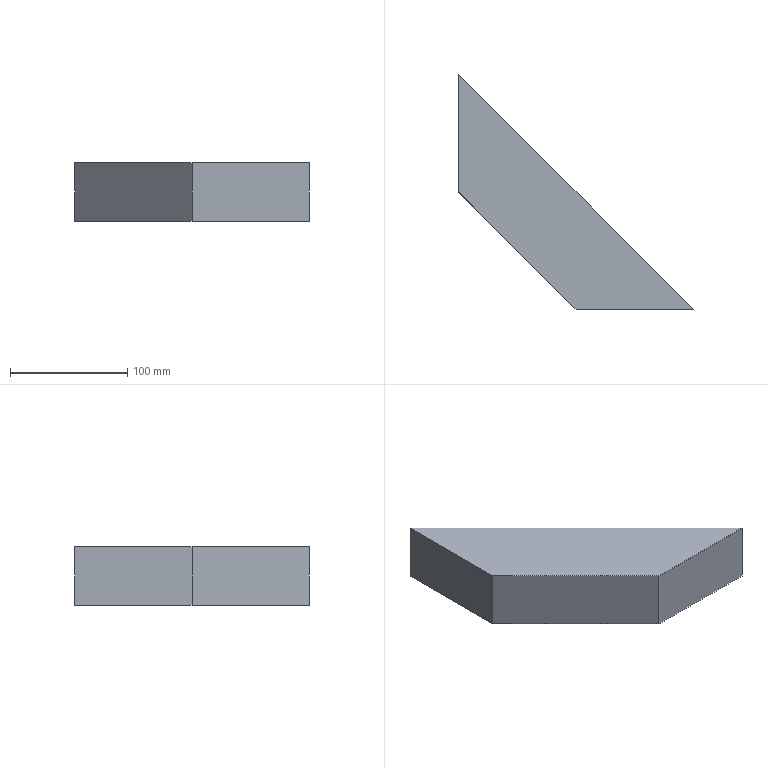Part | STEP file | Support rib 1 | 1 solid | 6 faces | box 200 x 200 x 50 mm | volume 750000 mm3 | plane 6
STEP:
#1=CARTESIAN_POINT('',(0.,100.,0.));
#2=VERTEX_POINT('',#1);
#3=CARTESIAN_POINT('',(100.,0.,0.));
#4=VERTEX_POINT('',#3);
#5=CARTESIAN_POINT('',(0.,100.,0.));
#6=DIRECTION('',(0.7071,-0.7071,0.));
#7=VECTOR('',#6,1000.);
#8=LINE('',#5,#7);
#9=EDGE_CURVE('',#2,#4,#8,.T.);
#10=ORIENTED_EDGE('',*,*,#9,.T.);
#11=CARTESIAN_POINT('',(100.,0.,50.));
#12=VERTEX_POINT('',#11);
#13=CARTESIAN_POINT('',(100.,0.,50.));
#14=DIRECTION('',(0.,0.,-1.));
#15=VECTOR('',#14,1000.);
#16=LINE('',#13,#15);
#17=EDGE_CURVE('',#12,#4,#16,.T.);
#18=ORIENTED_EDGE('',*,*,#17,.F.);
#19=CARTESIAN_POINT('',(0.,100.,50.));
#20=VERTEX_POINT('',#19);
#21=CARTESIAN_POINT('',(0.,100.,50.));
#22=DIRECTION('',(0.7071,-0.7071,0.));
#23=VECTOR('',#22,1000.);
#24=LINE('',#21,#23);
#25=EDGE_CURVE('',#20,#12,#24,.T.);
#26=ORIENTED_EDGE('',*,*,#25,.F.);
#27=CARTESIAN_POINT('',(0.,100.,50.));
#28=DIRECTION('',(0.,0.,-1.));
#29=VECTOR('',#28,1000.);
#30=LINE('',#27,#29);
#31=EDGE_CURVE('',#20,#2,#30,.T.);
#32=ORIENTED_EDGE('',*,*,#31,.T.);
#33=EDGE_LOOP('',(#10,#18,#26,#32));
#34=FACE_OUTER_BOUND('',#33,.T.);
#35=CARTESIAN_POINT('',(0.,100.,50.));
#36=DIRECTION('',(0.7071,0.7071,0.));
#37=DIRECTION('',(-0.7071,0.7071,0.));
#38=AXIS2_PLACEMENT_3D('',#35,#36,#37);
#39=PLANE('',#38);
#40=ADVANCED_FACE('',(#34),#39,.F.);
#41=CARTESIAN_POINT('',(200.,0.,0.));
#42=VERTEX_POINT('',#41);
#43=CARTESIAN_POINT('',(100.,0.,0.));
#44=DIRECTION('',(1.,0.,0.));
#45=VECTOR('',#44,1000.);
#46=LINE('',#43,#45);
#47=EDGE_CURVE('',#4,#42,#46,.T.);
#48=ORIENTED_EDGE('',*,*,#47,.T.);
#49=CARTESIAN_POINT('',(200.,0.,50.));
#50=VERTEX_POINT('',#49);
#51=CARTESIAN_POINT('',(200.,0.,50.));
#52=DIRECTION('',(0.,0.,-1.));
#53=VECTOR('',#52,1000.);
#54=LINE('',#51,#53);
#55=EDGE_CURVE('',#50,#42,#54,.T.);
#56=ORIENTED_EDGE('',*,*,#55,.F.);
#57=CARTESIAN_POINT('',(100.,0.,50.));
#58=DIRECTION('',(1.,0.,0.));
#59=VECTOR('',#58,1000.);
#60=LINE('',#57,#59);
#61=EDGE_CURVE('',#12,#50,#60,.T.);
#62=ORIENTED_EDGE('',*,*,#61,.F.);
#63=ORIENTED_EDGE('',*,*,#17,.T.);
#64=EDGE_LOOP('',(#48,#56,#62,#63));
#65=FACE_OUTER_BOUND('',#64,.T.);
#66=CARTESIAN_POINT('',(100.,0.,50.));
#67=DIRECTION('',(0.,1.,0.));
#68=DIRECTION('',(0.,0.,1.));
#69=AXIS2_PLACEMENT_3D('',#66,#67,#68);
#70=PLANE('',#69);
#71=ADVANCED_FACE('',(#65),#70,.F.);
#72=CARTESIAN_POINT('',(0.,200.,0.));
#73=VERTEX_POINT('',#72);
#74=CARTESIAN_POINT('',(0.,200.,0.));
#75=DIRECTION('',(-0.7071,0.7071,0.));
#76=VECTOR('',#75,1000.);
#77=LINE('',#74,#76);
#78=EDGE_CURVE('',#42,#73,#77,.T.);
#79=ORIENTED_EDGE('',*,*,#78,.T.);
#80=CARTESIAN_POINT('',(0.,200.,50.));
#81=VERTEX_POINT('',#80);
#82=CARTESIAN_POINT('',(0.,200.,50.));
#83=DIRECTION('',(0.,0.,-1.));
#84=VECTOR('',#83,1000.);
#85=LINE('',#82,#84);
#86=EDGE_CURVE('',#81,#73,#85,.T.);
#87=ORIENTED_EDGE('',*,*,#86,.F.);
#88=CARTESIAN_POINT('',(0.,200.,50.));
#89=DIRECTION('',(-0.7071,0.7071,0.));
#90=VECTOR('',#89,1000.);
#91=LINE('',#88,#90);
#92=EDGE_CURVE('',#50,#81,#91,.T.);
#93=ORIENTED_EDGE('',*,*,#92,.F.);
#94=ORIENTED_EDGE('',*,*,#55,.T.);
#95=EDGE_LOOP('',(#79,#87,#93,#94));
#96=FACE_OUTER_BOUND('',#95,.T.);
#97=CARTESIAN_POINT('',(0.,200.,50.));
#98=DIRECTION('',(-0.7071,-0.7071,0.));
#99=DIRECTION('',(0.7071,-0.7071,0.));
#100=AXIS2_PLACEMENT_3D('',#97,#98,#99);
#101=PLANE('',#100);
#102=ADVANCED_FACE('',(#96),#101,.F.);
#103=CARTESIAN_POINT('',(0.,100.,0.));
#104=DIRECTION('',(0.,-1.,0.));
#105=VECTOR('',#104,1000.);
#106=LINE('',#103,#105);
#107=EDGE_CURVE('',#73,#2,#106,.T.);
#108=ORIENTED_EDGE('',*,*,#107,.T.);
#109=ORIENTED_EDGE('',*,*,#31,.F.);
#110=CARTESIAN_POINT('',(0.,100.,50.));
#111=DIRECTION('',(0.,-1.,0.));
#112=VECTOR('',#111,1000.);
#113=LINE('',#110,#112);
#114=EDGE_CURVE('',#81,#20,#113,.T.);
#115=ORIENTED_EDGE('',*,*,#114,.F.);
#116=ORIENTED_EDGE('',*,*,#86,.T.);
#117=EDGE_LOOP('',(#108,#109,#115,#116));
#118=FACE_OUTER_BOUND('',#117,.T.);
#119=CARTESIAN_POINT('',(0.,100.,50.));
#120=DIRECTION('',(1.,0.,0.));
#121=DIRECTION('',(0.,0.,-1.));
#122=AXIS2_PLACEMENT_3D('',#119,#120,#121);
#123=PLANE('',#122);
#124=ADVANCED_FACE('',(#118),#123,.F.);
#125=ORIENTED_EDGE('',*,*,#25,.T.);
#126=ORIENTED_EDGE('',*,*,#61,.T.);
#127=ORIENTED_EDGE('',*,*,#92,.T.);
#128=ORIENTED_EDGE('',*,*,#114,.T.);
#129=EDGE_LOOP('',(#125,#126,#127,#128));
#130=FACE_OUTER_BOUND('',#129,.T.);
#131=CARTESIAN_POINT('',(0.,0.,50.));
#132=DIRECTION('',(0.,0.,1.));
#133=DIRECTION('',(1.,0.,0.));
#134=AXIS2_PLACEMENT_3D('',#131,#132,#133);
#135=PLANE('',#134);
#136=ADVANCED_FACE('',(#130),#135,.T.);
#137=ORIENTED_EDGE('',*,*,#9,.F.);
#138=ORIENTED_EDGE('',*,*,#107,.F.);
#139=ORIENTED_EDGE('',*,*,#78,.F.);
#140=ORIENTED_EDGE('',*,*,#47,.F.);
#141=EDGE_LOOP('',(#137,#138,#139,#140));
#142=FACE_OUTER_BOUND('',#141,.T.);
#143=CARTESIAN_POINT('',(0.,0.,0.));
#144=DIRECTION('',(0.,0.,1.));
#145=DIRECTION('',(1.,0.,0.));
#146=AXIS2_PLACEMENT_3D('',#143,#144,#145);
#147=PLANE('',#146);
#148=ADVANCED_FACE('',(#142),#147,.F.);
#149=CLOSED_SHELL('',(#40,#71,#102,#124,#136,#148));
#150=MANIFOLD_SOLID_BREP('',#149);
#151=CARTESIAN_POINT('',(0.,0.,0.));
#152=DIRECTION('',(0.,0.,1.));
#153=DIRECTION('',(1.,0.,0.));
#154=AXIS2_PLACEMENT_3D('',#151,#152,#153);
#155=(LENGTH_UNIT()NAMED_UNIT(*)SI_UNIT(.MILLI.,.METRE.));
#156=UNCERTAINTY_MEASURE_WITH_UNIT(LENGTH_MEASURE(0.00001),#155,'','');
#157=(NAMED_UNIT(*)PLANE_ANGLE_UNIT()SI_UNIT($,.RADIAN.));
#158=(NAMED_UNIT(*)SI_UNIT($,.STERADIAN.)SOLID_ANGLE_UNIT());
#159=(GEOMETRIC_REPRESENTATION_CONTEXT(3)GLOBAL_UNCERTAINTY_ASSIGNED_CONTEXT((#156))GLOBAL_UNIT_ASSIGNED_CONTEXT((#155,#157,#158))REPRESENTATION_CONTEXT('',''));
#160=ADVANCED_BREP_SHAPE_REPRESENTATION('',(#150,#154),#159);